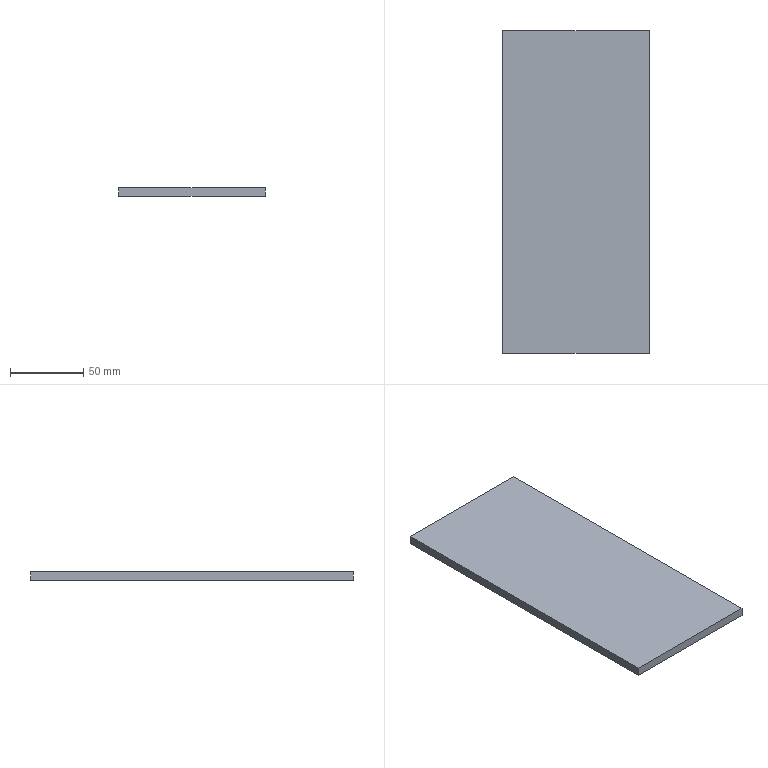Part | SolidWorks | features Extrusion 1 | 1 solid | 6 faces | box 100 x 220 x 6 mm | volume 132000 mm3 | plane 6
STEP:
#1=CARTESIAN_POINT('',(50.,-110.,0.));
#2=VERTEX_POINT('',#1);
#3=CARTESIAN_POINT('',(50.,110.,0.));
#4=VERTEX_POINT('',#3);
#5=CARTESIAN_POINT('',(50.,110.,0.));
#6=DIRECTION('',(0.,1.,0.));
#7=VECTOR('',#6,1000.);
#8=LINE('',#5,#7);
#9=EDGE_CURVE('',#2,#4,#8,.T.);
#10=ORIENTED_EDGE('',*,*,#9,.T.);
#11=CARTESIAN_POINT('',(50.,110.,6.));
#12=VERTEX_POINT('',#11);
#13=CARTESIAN_POINT('',(50.,110.,6.));
#14=DIRECTION('',(0.,0.,-1.));
#15=VECTOR('',#14,1000.);
#16=LINE('',#13,#15);
#17=EDGE_CURVE('',#12,#4,#16,.T.);
#18=ORIENTED_EDGE('',*,*,#17,.F.);
#19=CARTESIAN_POINT('',(50.,-110.,6.));
#20=VERTEX_POINT('',#19);
#21=CARTESIAN_POINT('',(50.,110.,6.));
#22=DIRECTION('',(0.,1.,0.));
#23=VECTOR('',#22,1000.);
#24=LINE('',#21,#23);
#25=EDGE_CURVE('',#20,#12,#24,.T.);
#26=ORIENTED_EDGE('',*,*,#25,.F.);
#27=CARTESIAN_POINT('',(50.,-110.,6.));
#28=DIRECTION('',(0.,0.,-1.));
#29=VECTOR('',#28,1000.);
#30=LINE('',#27,#29);
#31=EDGE_CURVE('',#20,#2,#30,.T.);
#32=ORIENTED_EDGE('',*,*,#31,.T.);
#33=EDGE_LOOP('',(#10,#18,#26,#32));
#34=FACE_OUTER_BOUND('',#33,.T.);
#35=CARTESIAN_POINT('',(50.,110.,6.));
#36=DIRECTION('',(-1.,0.,0.));
#37=DIRECTION('',(0.,-1.,0.));
#38=AXIS2_PLACEMENT_3D('',#35,#36,#37);
#39=PLANE('',#38);
#40=ADVANCED_FACE('',(#34),#39,.F.);
#41=CARTESIAN_POINT('',(-50.,110.,0.));
#42=VERTEX_POINT('',#41);
#43=CARTESIAN_POINT('',(-50.,110.,0.));
#44=DIRECTION('',(-1.,0.,0.));
#45=VECTOR('',#44,1000.);
#46=LINE('',#43,#45);
#47=EDGE_CURVE('',#4,#42,#46,.T.);
#48=ORIENTED_EDGE('',*,*,#47,.T.);
#49=CARTESIAN_POINT('',(-50.,110.,6.));
#50=VERTEX_POINT('',#49);
#51=CARTESIAN_POINT('',(-50.,110.,6.));
#52=DIRECTION('',(0.,0.,-1.));
#53=VECTOR('',#52,1000.);
#54=LINE('',#51,#53);
#55=EDGE_CURVE('',#50,#42,#54,.T.);
#56=ORIENTED_EDGE('',*,*,#55,.F.);
#57=CARTESIAN_POINT('',(-50.,110.,6.));
#58=DIRECTION('',(-1.,0.,0.));
#59=VECTOR('',#58,1000.);
#60=LINE('',#57,#59);
#61=EDGE_CURVE('',#12,#50,#60,.T.);
#62=ORIENTED_EDGE('',*,*,#61,.F.);
#63=ORIENTED_EDGE('',*,*,#17,.T.);
#64=EDGE_LOOP('',(#48,#56,#62,#63));
#65=FACE_OUTER_BOUND('',#64,.T.);
#66=CARTESIAN_POINT('',(-50.,110.,6.));
#67=DIRECTION('',(0.,-1.,0.));
#68=DIRECTION('',(0.,0.,-1.));
#69=AXIS2_PLACEMENT_3D('',#66,#67,#68);
#70=PLANE('',#69);
#71=ADVANCED_FACE('',(#65),#70,.F.);
#72=CARTESIAN_POINT('',(-50.,-110.,0.));
#73=VERTEX_POINT('',#72);
#74=CARTESIAN_POINT('',(-50.,110.,0.));
#75=DIRECTION('',(0.,-1.,0.));
#76=VECTOR('',#75,1000.);
#77=LINE('',#74,#76);
#78=EDGE_CURVE('',#42,#73,#77,.T.);
#79=ORIENTED_EDGE('',*,*,#78,.T.);
#80=CARTESIAN_POINT('',(-50.,-110.,6.));
#81=VERTEX_POINT('',#80);
#82=CARTESIAN_POINT('',(-50.,-110.,6.));
#83=DIRECTION('',(0.,0.,-1.));
#84=VECTOR('',#83,1000.);
#85=LINE('',#82,#84);
#86=EDGE_CURVE('',#81,#73,#85,.T.);
#87=ORIENTED_EDGE('',*,*,#86,.F.);
#88=CARTESIAN_POINT('',(-50.,110.,6.));
#89=DIRECTION('',(0.,-1.,0.));
#90=VECTOR('',#89,1000.);
#91=LINE('',#88,#90);
#92=EDGE_CURVE('',#50,#81,#91,.T.);
#93=ORIENTED_EDGE('',*,*,#92,.F.);
#94=ORIENTED_EDGE('',*,*,#55,.T.);
#95=EDGE_LOOP('',(#79,#87,#93,#94));
#96=FACE_OUTER_BOUND('',#95,.T.);
#97=CARTESIAN_POINT('',(-50.,110.,6.));
#98=DIRECTION('',(1.,0.,0.));
#99=DIRECTION('',(0.,1.,0.));
#100=AXIS2_PLACEMENT_3D('',#97,#98,#99);
#101=PLANE('',#100);
#102=ADVANCED_FACE('',(#96),#101,.F.);
#103=CARTESIAN_POINT('',(-50.,-110.,0.));
#104=DIRECTION('',(1.,0.,0.));
#105=VECTOR('',#104,1000.);
#106=LINE('',#103,#105);
#107=EDGE_CURVE('',#73,#2,#106,.T.);
#108=ORIENTED_EDGE('',*,*,#107,.T.);
#109=ORIENTED_EDGE('',*,*,#31,.F.);
#110=CARTESIAN_POINT('',(-50.,-110.,6.));
#111=DIRECTION('',(1.,0.,0.));
#112=VECTOR('',#111,1000.);
#113=LINE('',#110,#112);
#114=EDGE_CURVE('',#81,#20,#113,.T.);
#115=ORIENTED_EDGE('',*,*,#114,.F.);
#116=ORIENTED_EDGE('',*,*,#86,.T.);
#117=EDGE_LOOP('',(#108,#109,#115,#116));
#118=FACE_OUTER_BOUND('',#117,.T.);
#119=CARTESIAN_POINT('',(-50.,-110.,6.));
#120=DIRECTION('',(0.,1.,0.));
#121=DIRECTION('',(0.,0.,1.));
#122=AXIS2_PLACEMENT_3D('',#119,#120,#121);
#123=PLANE('',#122);
#124=ADVANCED_FACE('',(#118),#123,.F.);
#125=ORIENTED_EDGE('',*,*,#25,.T.);
#126=ORIENTED_EDGE('',*,*,#61,.T.);
#127=ORIENTED_EDGE('',*,*,#92,.T.);
#128=ORIENTED_EDGE('',*,*,#114,.T.);
#129=EDGE_LOOP('',(#125,#126,#127,#128));
#130=FACE_OUTER_BOUND('',#129,.T.);
#131=CARTESIAN_POINT('',(0.,0.,6.));
#132=DIRECTION('',(0.,0.,1.));
#133=DIRECTION('',(1.,0.,0.));
#134=AXIS2_PLACEMENT_3D('',#131,#132,#133);
#135=PLANE('',#134);
#136=ADVANCED_FACE('',(#130),#135,.T.);
#137=ORIENTED_EDGE('',*,*,#9,.F.);
#138=ORIENTED_EDGE('',*,*,#107,.F.);
#139=ORIENTED_EDGE('',*,*,#78,.F.);
#140=ORIENTED_EDGE('',*,*,#47,.F.);
#141=EDGE_LOOP('',(#137,#138,#139,#140));
#142=FACE_OUTER_BOUND('',#141,.T.);
#143=CARTESIAN_POINT('',(0.,0.,0.));
#144=DIRECTION('',(0.,0.,1.));
#145=DIRECTION('',(1.,0.,0.));
#146=AXIS2_PLACEMENT_3D('',#143,#144,#145);
#147=PLANE('',#146);
#148=ADVANCED_FACE('',(#142),#147,.F.);
#149=CLOSED_SHELL('',(#40,#71,#102,#124,#136,#148));
#150=MANIFOLD_SOLID_BREP('',#149);
#151=CARTESIAN_POINT('',(0.,0.,0.));
#152=DIRECTION('',(0.,0.,1.));
#153=DIRECTION('',(1.,0.,0.));
#154=AXIS2_PLACEMENT_3D('',#151,#152,#153);
#155=(LENGTH_UNIT()NAMED_UNIT(*)SI_UNIT(.MILLI.,.METRE.));
#156=UNCERTAINTY_MEASURE_WITH_UNIT(LENGTH_MEASURE(0.00001),#155,'','');
#157=(NAMED_UNIT(*)PLANE_ANGLE_UNIT()SI_UNIT($,.RADIAN.));
#158=(NAMED_UNIT(*)SI_UNIT($,.STERADIAN.)SOLID_ANGLE_UNIT());
#159=(GEOMETRIC_REPRESENTATION_CONTEXT(3)GLOBAL_UNCERTAINTY_ASSIGNED_CONTEXT((#156))GLOBAL_UNIT_ASSIGNED_CONTEXT((#155,#157,#158))REPRESENTATION_CONTEXT('',''));
#160=ADVANCED_BREP_SHAPE_REPRESENTATION('',(#150,#154),#159);